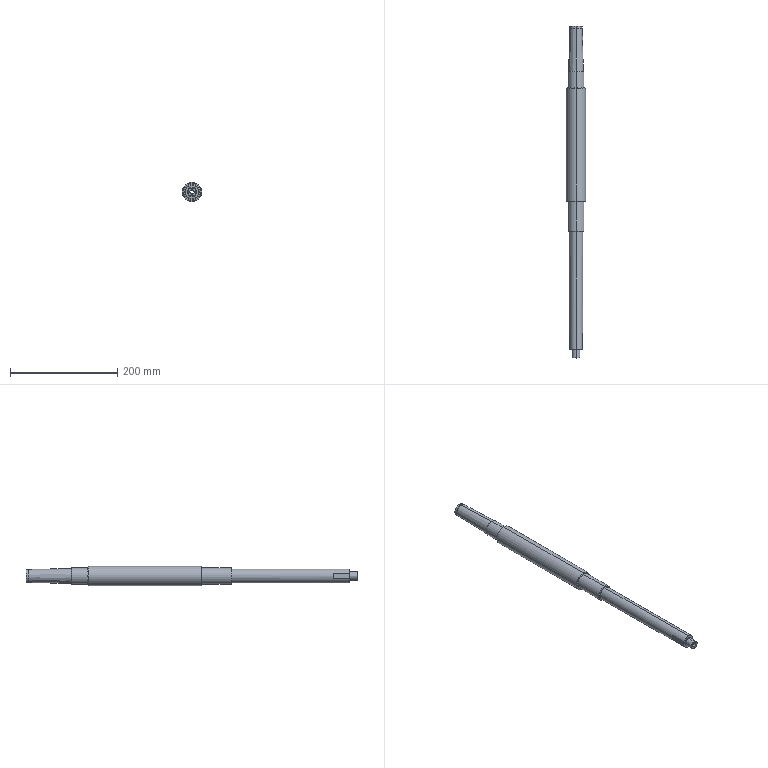Part | NX | features BREP 1 | 1 solid | 51 faces | box 36 x 618 x 36 mm | volume 396919 mm3 | cylinder 21 | plane 16 | torus 10 | cone 4 | commonest cylinder face diameters 8 x5 30 x4 14.5 x2 15 x2 22 x2 24 x2
STEP:
#1=CARTESIAN_POINT('',(0.,137.,14.975));
#2=VERTEX_POINT('',#1);
#3=CARTESIAN_POINT('',(0.,137.,-14.975));
#4=VERTEX_POINT('',#3);
#5=CARTESIAN_POINT('',(0.,137.,0.));
#6=DIRECTION('',(0.,-1.,0.));
#7=DIRECTION('',(0.,0.,-1.));
#8=AXIS2_PLACEMENT_3D('',#5,#6,#7);
#9=CIRCLE('',#8,14.975);
#10=EDGE_CURVE('',#2,#4,#9,.T.);
#11=ORIENTED_EDGE('',*,*,#10,.F.);
#12=CARTESIAN_POINT('',(0.,137.975,13.976));
#13=VERTEX_POINT('',#12);
#14=CARTESIAN_POINT('',(0.,138.,14.975));
#15=DIRECTION('',(1.,0.,0.));
#16=DIRECTION('',(0.,0.,-1.));
#17=AXIS2_PLACEMENT_3D('',#14,#15,#16);
#18=CIRCLE('',#17,1.);
#19=EDGE_CURVE('',#13,#2,#18,.F.);
#20=ORIENTED_EDGE('',*,*,#19,.F.);
#21=CARTESIAN_POINT('',(0.,137.975,-13.976));
#22=VERTEX_POINT('',#21);
#23=CARTESIAN_POINT('',(0.,137.975,0.));
#24=DIRECTION('',(0.,1.,0.));
#25=DIRECTION('',(0.,0.,-1.));
#26=AXIS2_PLACEMENT_3D('',#23,#24,#25);
#27=CIRCLE('',#26,13.976);
#28=EDGE_CURVE('',#22,#13,#27,.T.);
#29=ORIENTED_EDGE('',*,*,#28,.F.);
#30=CARTESIAN_POINT('',(0.,138.,-14.975));
#31=DIRECTION('',(-1.,0.,0.));
#32=DIRECTION('',(0.,-1.,0.));
#33=AXIS2_PLACEMENT_3D('',#30,#31,#32);
#34=CIRCLE('',#33,1.);
#35=EDGE_CURVE('',#22,#4,#34,.F.);
#36=ORIENTED_EDGE('',*,*,#35,.T.);
#37=EDGE_LOOP('',(#11,#20,#29,#36));
#38=FACE_BOUND('',#37,.T.);
#39=CARTESIAN_POINT('',(0.,138.,0.));
#40=DIRECTION('',(0.,-1.,0.));
#41=DIRECTION('',(0.,0.,1.));
#42=AXIS2_PLACEMENT_3D('',#39,#40,#41);
#43=TOROIDAL_SURFACE('',#42,14.975,1.);
#44=ADVANCED_FACE('',(#38),#43,.F.);
#45=CARTESIAN_POINT('',(0.,106.,16.));
#46=VERTEX_POINT('',#45);
#47=CARTESIAN_POINT('',(0.,106.,-16.));
#48=VERTEX_POINT('',#47);
#49=CARTESIAN_POINT('',(0.,106.,0.));
#50=DIRECTION('',(0.,-1.,0.));
#51=DIRECTION('',(0.,0.,-1.));
#52=AXIS2_PLACEMENT_3D('',#49,#50,#51);
#53=CIRCLE('',#52,16.);
#54=EDGE_CURVE('',#46,#48,#53,.T.);
#55=ORIENTED_EDGE('',*,*,#54,.F.);
#56=CARTESIAN_POINT('',(0.,107.,15.));
#57=VERTEX_POINT('',#56);
#58=CARTESIAN_POINT('',(0.,107.,16.));
#59=DIRECTION('',(1.,0.,0.));
#60=DIRECTION('',(0.,0.,-1.));
#61=AXIS2_PLACEMENT_3D('',#58,#59,#60);
#62=CIRCLE('',#61,1.);
#63=EDGE_CURVE('',#57,#46,#62,.F.);
#64=ORIENTED_EDGE('',*,*,#63,.F.);
#65=CARTESIAN_POINT('',(0.,107.,-15.));
#66=VERTEX_POINT('',#65);
#67=CARTESIAN_POINT('',(0.,107.,0.));
#68=DIRECTION('',(0.,1.,0.));
#69=DIRECTION('',(0.,0.,-1.));
#70=AXIS2_PLACEMENT_3D('',#67,#68,#69);
#71=CIRCLE('',#70,15.);
#72=EDGE_CURVE('',#66,#57,#71,.T.);
#73=ORIENTED_EDGE('',*,*,#72,.F.);
#74=CARTESIAN_POINT('',(0.,107.,-16.));
#75=DIRECTION('',(-1.,0.,0.));
#76=DIRECTION('',(0.,-1.,0.));
#77=AXIS2_PLACEMENT_3D('',#74,#75,#76);
#78=CIRCLE('',#77,1.);
#79=EDGE_CURVE('',#66,#48,#78,.F.);
#80=ORIENTED_EDGE('',*,*,#79,.T.);
#81=EDGE_LOOP('',(#55,#64,#73,#80));
#82=FACE_BOUND('',#81,.T.);
#83=CARTESIAN_POINT('',(0.,107.,0.));
#84=DIRECTION('',(0.,-1.,0.));
#85=DIRECTION('',(0.,0.,1.));
#86=AXIS2_PLACEMENT_3D('',#83,#84,#85);
#87=TOROIDAL_SURFACE('',#86,16.,1.);
#88=ADVANCED_FACE('',(#82),#87,.F.);
#89=CARTESIAN_POINT('',(0.,-104.,-16.));
#90=VERTEX_POINT('',#89);
#91=CARTESIAN_POINT('',(0.,-104.,16.));
#92=VERTEX_POINT('',#91);
#93=CARTESIAN_POINT('',(0.,-104.,0.));
#94=DIRECTION('',(0.,1.,0.));
#95=DIRECTION('',(0.,0.,1.));
#96=AXIS2_PLACEMENT_3D('',#93,#94,#95);
#97=CIRCLE('',#96,16.);
#98=EDGE_CURVE('',#90,#92,#97,.T.);
#99=ORIENTED_EDGE('',*,*,#98,.F.);
#100=CARTESIAN_POINT('',(0.,-105.,-15.));
#101=VERTEX_POINT('',#100);
#102=CARTESIAN_POINT('',(0.,-105.,-16.));
#103=DIRECTION('',(1.,0.,0.));
#104=DIRECTION('',(0.,0.,-1.));
#105=AXIS2_PLACEMENT_3D('',#102,#103,#104);
#106=CIRCLE('',#105,1.);
#107=EDGE_CURVE('',#90,#101,#106,.T.);
#108=ORIENTED_EDGE('',*,*,#107,.T.);
#109=CARTESIAN_POINT('',(0.,-105.,15.));
#110=VERTEX_POINT('',#109);
#111=CARTESIAN_POINT('',(0.,-105.,0.));
#112=DIRECTION('',(0.,-1.,0.));
#113=DIRECTION('',(0.,0.,1.));
#114=AXIS2_PLACEMENT_3D('',#111,#112,#113);
#115=CIRCLE('',#114,15.);
#116=EDGE_CURVE('',#110,#101,#115,.T.);
#117=ORIENTED_EDGE('',*,*,#116,.F.);
#118=CARTESIAN_POINT('',(0.,-105.,16.));
#119=DIRECTION('',(-1.,0.,0.));
#120=DIRECTION('',(0.,-1.,0.));
#121=AXIS2_PLACEMENT_3D('',#118,#119,#120);
#122=CIRCLE('',#121,1.);
#123=EDGE_CURVE('',#92,#110,#122,.T.);
#124=ORIENTED_EDGE('',*,*,#123,.F.);
#125=EDGE_LOOP('',(#99,#108,#117,#124));
#126=FACE_BOUND('',#125,.T.);
#127=CARTESIAN_POINT('',(0.,-105.,0.));
#128=DIRECTION('',(0.,1.,0.));
#129=DIRECTION('',(0.,0.,-1.));
#130=AXIS2_PLACEMENT_3D('',#127,#128,#129);
#131=TOROIDAL_SURFACE('',#130,16.,1.);
#132=ADVANCED_FACE('',(#126),#131,.F.);
#133=CARTESIAN_POINT('',(0.,-160.,-13.5));
#134=VERTEX_POINT('',#133);
#135=CARTESIAN_POINT('',(0.,-160.,13.5));
#136=VERTEX_POINT('',#135);
#137=CARTESIAN_POINT('',(0.,-160.,0.));
#138=DIRECTION('',(0.,1.,0.));
#139=DIRECTION('',(0.,0.,1.));
#140=AXIS2_PLACEMENT_3D('',#137,#138,#139);
#141=CIRCLE('',#140,13.5);
#142=EDGE_CURVE('',#134,#136,#141,.T.);
#143=ORIENTED_EDGE('',*,*,#142,.F.);
#144=CARTESIAN_POINT('',(0.,-161.,-12.5));
#145=VERTEX_POINT('',#144);
#146=CARTESIAN_POINT('',(0.,-161.,-13.5));
#147=DIRECTION('',(1.,0.,0.));
#148=DIRECTION('',(0.,0.,-1.));
#149=AXIS2_PLACEMENT_3D('',#146,#147,#148);
#150=CIRCLE('',#149,1.);
#151=EDGE_CURVE('',#134,#145,#150,.T.);
#152=ORIENTED_EDGE('',*,*,#151,.T.);
#153=CARTESIAN_POINT('',(0.,-161.,12.5));
#154=VERTEX_POINT('',#153);
#155=CARTESIAN_POINT('',(0.,-161.,0.));
#156=DIRECTION('',(0.,-1.,0.));
#157=DIRECTION('',(0.,0.,1.));
#158=AXIS2_PLACEMENT_3D('',#155,#156,#157);
#159=CIRCLE('',#158,12.5);
#160=EDGE_CURVE('',#154,#145,#159,.T.);
#161=ORIENTED_EDGE('',*,*,#160,.F.);
#162=CARTESIAN_POINT('',(0.,-161.,13.5));
#163=DIRECTION('',(-1.,0.,0.));
#164=DIRECTION('',(0.,-1.,0.));
#165=AXIS2_PLACEMENT_3D('',#162,#163,#164);
#166=CIRCLE('',#165,1.);
#167=EDGE_CURVE('',#136,#154,#166,.T.);
#168=ORIENTED_EDGE('',*,*,#167,.F.);
#169=EDGE_LOOP('',(#143,#152,#161,#168));
#170=FACE_BOUND('',#169,.T.);
#171=CARTESIAN_POINT('',(0.,-161.,0.));
#172=DIRECTION('',(0.,1.,0.));
#173=DIRECTION('',(0.,0.,-1.));
#174=AXIS2_PLACEMENT_3D('',#171,#172,#173);
#175=TOROIDAL_SURFACE('',#174,13.5,1.);
#176=ADVANCED_FACE('',(#170),#175,.F.);
#177=CARTESIAN_POINT('',(0.,-380.,-8.5));
#178=VERTEX_POINT('',#177);
#179=CARTESIAN_POINT('',(0.,-380.,8.5));
#180=VERTEX_POINT('',#179);
#181=CARTESIAN_POINT('',(0.,-380.,0.));
#182=DIRECTION('',(0.,1.,0.));
#183=DIRECTION('',(0.,0.,1.));
#184=AXIS2_PLACEMENT_3D('',#181,#182,#183);
#185=CIRCLE('',#184,8.5);
#186=EDGE_CURVE('',#178,#180,#185,.T.);
#187=ORIENTED_EDGE('',*,*,#186,.F.);
#188=CARTESIAN_POINT('',(0.,-381.,-7.5));
#189=VERTEX_POINT('',#188);
#190=CARTESIAN_POINT('',(0.,-381.,-8.5));
#191=DIRECTION('',(1.,0.,0.));
#192=DIRECTION('',(0.,0.,-1.));
#193=AXIS2_PLACEMENT_3D('',#190,#191,#192);
#194=CIRCLE('',#193,1.);
#195=EDGE_CURVE('',#178,#189,#194,.T.);
#196=ORIENTED_EDGE('',*,*,#195,.T.);
#197=CARTESIAN_POINT('',(0.,-381.,7.5));
#198=VERTEX_POINT('',#197);
#199=CARTESIAN_POINT('',(0.,-381.,0.));
#200=DIRECTION('',(0.,-1.,0.));
#201=DIRECTION('',(0.,0.,1.));
#202=AXIS2_PLACEMENT_3D('',#199,#200,#201);
#203=CIRCLE('',#202,7.5);
#204=EDGE_CURVE('',#198,#189,#203,.T.);
#205=ORIENTED_EDGE('',*,*,#204,.F.);
#206=CARTESIAN_POINT('',(0.,-381.,8.5));
#207=DIRECTION('',(-1.,0.,0.));
#208=DIRECTION('',(0.,-1.,0.));
#209=AXIS2_PLACEMENT_3D('',#206,#207,#208);
#210=CIRCLE('',#209,1.);
#211=EDGE_CURVE('',#180,#198,#210,.T.);
#212=ORIENTED_EDGE('',*,*,#211,.F.);
#213=EDGE_LOOP('',(#187,#196,#205,#212));
#214=FACE_BOUND('',#213,.T.);
#215=CARTESIAN_POINT('',(0.,-381.,0.));
#216=DIRECTION('',(0.,1.,0.));
#217=DIRECTION('',(0.,0.,-1.));
#218=AXIS2_PLACEMENT_3D('',#215,#216,#217);
#219=TOROIDAL_SURFACE('',#218,8.5,1.);
#220=ADVANCED_FACE('',(#214),#219,.F.);
#221=CARTESIAN_POINT('',(12.763,162.,4.));
#222=VERTEX_POINT('',#221);
#223=CARTESIAN_POINT('',(13.475,158.,0.));
#224=VERTEX_POINT('',#223);
#225=CARTESIAN_POINT('',(12.763,162.,4.));
#226=CARTESIAN_POINT('',(12.791,160.935,4.));
#227=CARTESIAN_POINT('',(13.156,158.88,3.129));
#228=CARTESIAN_POINT('',(13.475,158.,1.065));
#229=CARTESIAN_POINT('',(13.475,158.,0.));
#230=B_SPLINE_CURVE_WITH_KNOTS('',3,(#225,#226,#227,#228,#229),.UNSPECIFIED.,.F.,.F.,(4,1,4),(0.,0.003148,0.006296),.UNSPECIFIED.);
#231=EDGE_CURVE('',#222,#224,#230,.T.);
#232=ORIENTED_EDGE('',*,*,#231,.T.);
#233=CARTESIAN_POINT('',(8.4,158.,0.));
#234=VERTEX_POINT('',#233);
#235=CARTESIAN_POINT('',(21.,158.,0.));
#236=DIRECTION('',(-1.,0.,0.));
#237=VECTOR('',#236,1000.);
#238=LINE('',#235,#237);
#239=EDGE_CURVE('',#224,#234,#238,.T.);
#240=ORIENTED_EDGE('',*,*,#239,.T.);
#241=CARTESIAN_POINT('',(8.4,162.,4.));
#242=VERTEX_POINT('',#241);
#243=CARTESIAN_POINT('',(8.4,162.,0.));
#244=DIRECTION('',(1.,0.,0.));
#245=DIRECTION('',(0.,1.,0.));
#246=AXIS2_PLACEMENT_3D('',#243,#244,#245);
#247=CIRCLE('',#246,4.);
#248=EDGE_CURVE('',#242,#234,#247,.T.);
#249=ORIENTED_EDGE('',*,*,#248,.F.);
#250=CARTESIAN_POINT('',(11.,162.,4.));
#251=DIRECTION('',(1.,0.,0.));
#252=VECTOR('',#251,1000.);
#253=LINE('',#250,#252);
#254=EDGE_CURVE('',#242,#222,#253,.T.);
#255=ORIENTED_EDGE('',*,*,#254,.T.);
#256=EDGE_LOOP('',(#232,#240,#249,#255));
#257=FACE_BOUND('',#256,.T.);
#258=CARTESIAN_POINT('',(21.,162.,0.));
#259=DIRECTION('',(-1.,0.,0.));
#260=DIRECTION('',(0.,1.,0.));
#261=AXIS2_PLACEMENT_3D('',#258,#259,#260);
#262=CYLINDRICAL_SURFACE('',#261,4.);
#263=ADVANCED_FACE('',(#257),#262,.F.);
#264=CARTESIAN_POINT('',(0.,217.,11.));
#265=VERTEX_POINT('',#264);
#266=CARTESIAN_POINT('',(0.,217.,-11.));
#267=VERTEX_POINT('',#266);
#268=CARTESIAN_POINT('',(0.,217.,0.));
#269=DIRECTION('',(0.,1.,0.));
#270=DIRECTION('',(0.,0.,1.));
#271=AXIS2_PLACEMENT_3D('',#268,#269,#270);
#272=CIRCLE('',#271,11.);
#273=EDGE_CURVE('',#265,#267,#272,.T.);
#274=ORIENTED_EDGE('',*,*,#273,.T.);
#275=CARTESIAN_POINT('',(0.,218.,-11.));
#276=VERTEX_POINT('',#275);
#277=CARTESIAN_POINT('',(0.,217.,-11.));
#278=DIRECTION('',(0.,1.,0.));
#279=VECTOR('',#278,1000.);
#280=LINE('',#277,#279);
#281=EDGE_CURVE('',#267,#276,#280,.T.);
#282=ORIENTED_EDGE('',*,*,#281,.T.);
#283=CARTESIAN_POINT('',(0.,218.,11.));
#284=VERTEX_POINT('',#283);
#285=CARTESIAN_POINT('',(0.,218.,0.));
#286=DIRECTION('',(0.,1.,0.));
#287=DIRECTION('',(0.,0.,1.));
#288=AXIS2_PLACEMENT_3D('',#285,#286,#287);
#289=CIRCLE('',#288,11.);
#290=EDGE_CURVE('',#284,#276,#289,.T.);
#291=ORIENTED_EDGE('',*,*,#290,.F.);
#292=CARTESIAN_POINT('',(0.,217.,11.));
#293=DIRECTION('',(0.,1.,0.));
#294=VECTOR('',#293,1000.);
#295=LINE('',#292,#294);
#296=EDGE_CURVE('',#265,#284,#295,.T.);
#297=ORIENTED_EDGE('',*,*,#296,.F.);
#298=EDGE_LOOP('',(#274,#282,#291,#297));
#299=FACE_BOUND('',#298,.T.);
#300=CARTESIAN_POINT('',(0.,217.,0.));
#301=DIRECTION('',(0.,1.,0.));
#302=DIRECTION('',(0.,0.,-1.));
#303=AXIS2_PLACEMENT_3D('',#300,#301,#302);
#304=CYLINDRICAL_SURFACE('',#303,11.);
#305=ADVANCED_FACE('',(#299),#304,.T.);
#306=CARTESIAN_POINT('',(0.,212.,-8.038));
#307=VERTEX_POINT('',#306);
#308=CARTESIAN_POINT('',(0.,212.,6.462));
#309=VERTEX_POINT('',#308);
#310=CARTESIAN_POINT('',(0.,212.,-0.7881));
#311=DIRECTION('',(0.,1.,0.));
#312=DIRECTION('',(0.,0.,1.));
#313=AXIS2_PLACEMENT_3D('',#310,#311,#312);
#314=CIRCLE('',#313,7.25);
#315=EDGE_CURVE('',#307,#309,#314,.T.);
#316=ORIENTED_EDGE('',*,*,#315,.F.);
#317=CARTESIAN_POINT('',(0.,222.,-8.038));
#318=VERTEX_POINT('',#317);
#319=CARTESIAN_POINT('',(0.,222.,-8.038));
#320=DIRECTION('',(0.,1.,0.));
#321=VECTOR('',#320,1000.);
#322=LINE('',#319,#321);
#323=EDGE_CURVE('',#307,#318,#322,.T.);
#324=ORIENTED_EDGE('',*,*,#323,.T.);
#325=CARTESIAN_POINT('',(0.,222.,6.462));
#326=VERTEX_POINT('',#325);
#327=CARTESIAN_POINT('',(0.,222.,-0.7881));
#328=DIRECTION('',(0.,1.,0.));
#329=DIRECTION('',(0.,0.,1.));
#330=AXIS2_PLACEMENT_3D('',#327,#328,#329);
#331=CIRCLE('',#330,7.25);
#332=EDGE_CURVE('',#318,#326,#331,.T.);
#333=ORIENTED_EDGE('',*,*,#332,.T.);
#334=CARTESIAN_POINT('',(0.,222.,6.462));
#335=DIRECTION('',(0.,1.,0.));
#336=VECTOR('',#335,1000.);
#337=LINE('',#334,#336);
#338=EDGE_CURVE('',#309,#326,#337,.T.);
#339=ORIENTED_EDGE('',*,*,#338,.F.);
#340=EDGE_LOOP('',(#316,#324,#333,#339));
#341=FACE_BOUND('',#340,.T.);
#342=CARTESIAN_POINT('',(0.,222.,-0.7881));
#343=DIRECTION('',(0.,1.,0.));
#344=DIRECTION('',(0.,0.,-1.));
#345=AXIS2_PLACEMENT_3D('',#342,#343,#344);
#346=CYLINDRICAL_SURFACE('',#345,7.25);
#347=ADVANCED_FACE('',(#341),#346,.F.);
#348=CARTESIAN_POINT('',(0.,209.574,-4.));
#349=VERTEX_POINT('',#348);
#350=CARTESIAN_POINT('',(0.,210.521,4.));
#351=VERTEX_POINT('',#350);
#352=CARTESIAN_POINT('',(0.,209.574,-4.));
#353=CARTESIAN_POINT('',(-1.061,209.574,-4.));
#354=CARTESIAN_POINT('',(-3.135,209.707,-3.125));
#355=CARTESIAN_POINT('',(-4.431,210.103,-0.008504));
#356=CARTESIAN_POINT('',(-3.141,210.436,3.124));
#357=CARTESIAN_POINT('',(-1.061,210.521,4.));
#358=CARTESIAN_POINT('',(0.,210.521,4.));
#359=B_SPLINE_CURVE_WITH_KNOTS('',3,(#352,#353,#354,#355,#356,#357,#358),.UNSPECIFIED.,.F.,.F.,(4,1,1,1,4),(0.,0.003137,0.006274,0.009411,0.01255),.UNSPECIFIED.);
#360=EDGE_CURVE('',#349,#351,#359,.T.);
#361=ORIENTED_EDGE('',*,*,#360,.F.);
#362=CARTESIAN_POINT('',(0.,212.,-8.038));
#363=DIRECTION('',(0.,0.515,-0.8572));
#364=VECTOR('',#363,1000.);
#365=LINE('',#362,#364);
#366=EDGE_CURVE('',#349,#307,#365,.T.);
#367=ORIENTED_EDGE('',*,*,#366,.T.);
#368=ORIENTED_EDGE('',*,*,#315,.T.);
#369=CARTESIAN_POINT('',(0.,212.,6.462));
#370=DIRECTION('',(0.,0.515,0.8572));
#371=VECTOR('',#370,1000.);
#372=LINE('',#369,#371);
#373=EDGE_CURVE('',#351,#309,#372,.T.);
#374=ORIENTED_EDGE('',*,*,#373,.F.);
#375=EDGE_LOOP('',(#361,#367,#368,#374));
#376=FACE_BOUND('',#375,.T.);
#377=CARTESIAN_POINT('',(0.,212.,-0.7881));
#378=DIRECTION('',(0.,1.,0.));
#379=DIRECTION('',(0.,0.,-1.));
#380=AXIS2_PLACEMENT_3D('',#377,#378,#379);
#381=CONICAL_SURFACE('',#380,7.25,1.03);
#382=ADVANCED_FACE('',(#376),#381,.F.);
#383=CARTESIAN_POINT('',(0.,137.,-15.));
#384=VERTEX_POINT('',#383);
#385=CARTESIAN_POINT('',(0.,137.,15.));
#386=VERTEX_POINT('',#385);
#387=CARTESIAN_POINT('',(0.,137.,0.));
#388=DIRECTION('',(0.,-1.,0.));
#389=DIRECTION('',(0.,0.,-1.));
#390=AXIS2_PLACEMENT_3D('',#387,#388,#389);
#391=CIRCLE('',#390,15.);
#392=EDGE_CURVE('',#384,#386,#391,.T.);
#393=ORIENTED_EDGE('',*,*,#392,.T.);
#394=CARTESIAN_POINT('',(0.,0.,15.));
#395=DIRECTION('',(0.,-1.,0.));
#396=VECTOR('',#395,1000.);
#397=LINE('',#394,#396);
#398=EDGE_CURVE('',#57,#386,#397,.F.);
#399=ORIENTED_EDGE('',*,*,#398,.F.);
#400=CARTESIAN_POINT('',(0.,107.,0.));
#401=DIRECTION('',(0.,1.,0.));
#402=DIRECTION('',(0.,0.,-1.));
#403=AXIS2_PLACEMENT_3D('',#400,#401,#402);
#404=CIRCLE('',#403,15.);
#405=EDGE_CURVE('',#57,#66,#404,.T.);
#406=ORIENTED_EDGE('',*,*,#405,.T.);
#407=CARTESIAN_POINT('',(0.,0.,-15.));
#408=DIRECTION('',(0.,-1.,0.));
#409=VECTOR('',#408,1000.);
#410=LINE('',#407,#409);
#411=EDGE_CURVE('',#66,#384,#410,.F.);
#412=ORIENTED_EDGE('',*,*,#411,.T.);
#413=EDGE_LOOP('',(#393,#399,#406,#412));
#414=FACE_BOUND('',#413,.T.);
#415=CARTESIAN_POINT('',(0.,0.,0.));
#416=DIRECTION('',(0.,-1.,0.));
#417=DIRECTION('',(0.,0.,1.));
#418=AXIS2_PLACEMENT_3D('',#415,#416,#417);
#419=CYLINDRICAL_SURFACE('',#418,15.);
#420=ADVANCED_FACE('',(#414),#419,.T.);
#421=CARTESIAN_POINT('',(0.,222.,-12.));
#422=VERTEX_POINT('',#421);
#423=CARTESIAN_POINT('',(0.,222.,12.));
#424=VERTEX_POINT('',#423);
#425=CARTESIAN_POINT('',(0.,222.,0.));
#426=DIRECTION('',(0.,-1.,0.));
#427=DIRECTION('',(0.,0.,-1.));
#428=AXIS2_PLACEMENT_3D('',#425,#426,#427);
#429=CIRCLE('',#428,12.);
#430=EDGE_CURVE('',#422,#424,#429,.T.);
#431=ORIENTED_EDGE('',*,*,#430,.T.);
#432=CARTESIAN_POINT('',(0.,218.,12.));
#433=VERTEX_POINT('',#432);
#434=CARTESIAN_POINT('',(0.,0.,12.));
#435=DIRECTION('',(0.,-1.,0.));
#436=VECTOR('',#435,1000.);
#437=LINE('',#434,#436);
#438=EDGE_CURVE('',#433,#424,#437,.F.);
#439=ORIENTED_EDGE('',*,*,#438,.F.);
#440=CARTESIAN_POINT('',(0.,218.,-12.));
#441=VERTEX_POINT('',#440);
#442=CARTESIAN_POINT('',(0.,218.,0.));
#443=DIRECTION('',(0.,1.,0.));
#444=DIRECTION('',(0.,0.,1.));
#445=AXIS2_PLACEMENT_3D('',#442,#443,#444);
#446=CIRCLE('',#445,12.);
#447=EDGE_CURVE('',#433,#441,#446,.T.);
#448=ORIENTED_EDGE('',*,*,#447,.T.);
#449=CARTESIAN_POINT('',(0.,0.,-12.));
#450=DIRECTION('',(0.,-1.,0.));
#451=VECTOR('',#450,1000.);
#452=LINE('',#449,#451);
#453=EDGE_CURVE('',#441,#422,#452,.F.);
#454=ORIENTED_EDGE('',*,*,#453,.T.);
#455=EDGE_LOOP('',(#431,#439,#448,#454));
#456=FACE_BOUND('',#455,.T.);
#457=CARTESIAN_POINT('',(0.,0.,0.));
#458=DIRECTION('',(0.,-1.,0.));
#459=DIRECTION('',(0.,0.,1.));
#460=AXIS2_PLACEMENT_3D('',#457,#458,#459);
#461=CYLINDRICAL_SURFACE('',#460,12.);
#462=ADVANCED_FACE('',(#456),#461,.T.);
#463=ORIENTED_EDGE('',*,*,#360,.T.);
#464=CARTESIAN_POINT('',(0.,-396.,4.));
#465=VERTEX_POINT('',#464);
#466=CARTESIAN_POINT('',(0.,0.,4.));
#467=DIRECTION('',(0.,-1.,0.));
#468=VECTOR('',#467,1000.);
#469=LINE('',#466,#468);
#470=EDGE_CURVE('',#465,#351,#469,.F.);
#471=ORIENTED_EDGE('',*,*,#470,.F.);
#472=CARTESIAN_POINT('',(0.,-396.,-4.));
#473=VERTEX_POINT('',#472);
#474=CARTESIAN_POINT('',(0.,-396.,0.));
#475=DIRECTION('',(0.,-1.,0.));
#476=DIRECTION('',(0.,0.,-1.));
#477=AXIS2_PLACEMENT_3D('',#474,#475,#476);
#478=CIRCLE('',#477,4.);
#479=EDGE_CURVE('',#465,#473,#478,.T.);
#480=ORIENTED_EDGE('',*,*,#479,.T.);
#481=CARTESIAN_POINT('',(0.,0.,-4.));
#482=DIRECTION('',(0.,-1.,0.));
#483=VECTOR('',#482,1000.);
#484=LINE('',#481,#483);
#485=EDGE_CURVE('',#473,#349,#484,.F.);
#486=ORIENTED_EDGE('',*,*,#485,.T.);
#487=EDGE_LOOP('',(#463,#471,#480,#486));
#488=FACE_BOUND('',#487,.T.);
#489=CARTESIAN_POINT('',(0.,0.,0.));
#490=DIRECTION('',(0.,-1.,0.));
#491=DIRECTION('',(0.,0.,1.));
#492=AXIS2_PLACEMENT_3D('',#489,#490,#491);
#493=CYLINDRICAL_SURFACE('',#492,4.);
#494=ADVANCED_FACE('',(#488),#493,.F.);
#495=CARTESIAN_POINT('',(0.,-381.,0.));
#496=DIRECTION('',(0.,-1.,0.));
#497=DIRECTION('',(0.,0.,1.));
#498=AXIS2_PLACEMENT_3D('',#495,#496,#497);
#499=CIRCLE('',#498,7.5);
#500=EDGE_CURVE('',#189,#198,#499,.T.);
#501=ORIENTED_EDGE('',*,*,#500,.T.);
#502=CARTESIAN_POINT('',(0.,-396.,7.5));
#503=VERTEX_POINT('',#502);
#504=CARTESIAN_POINT('',(0.,0.,7.5));
#505=DIRECTION('',(0.,-1.,0.));
#506=VECTOR('',#505,1000.);
#507=LINE('',#504,#506);
#508=EDGE_CURVE('',#503,#198,#507,.F.);
#509=ORIENTED_EDGE('',*,*,#508,.F.);
#510=CARTESIAN_POINT('',(0.,-396.,-7.5));
#511=VERTEX_POINT('',#510);
#512=CARTESIAN_POINT('',(0.,-396.,0.));
#513=DIRECTION('',(0.,-1.,0.));
#514=DIRECTION('',(0.,0.,-1.));
#515=AXIS2_PLACEMENT_3D('',#512,#513,#514);
#516=CIRCLE('',#515,7.5);
#517=EDGE_CURVE('',#511,#503,#516,.T.);
#518=ORIENTED_EDGE('',*,*,#517,.F.);
#519=CARTESIAN_POINT('',(0.,0.,-7.5));
#520=DIRECTION('',(0.,-1.,0.));
#521=VECTOR('',#520,1000.);
#522=LINE('',#519,#521);
#523=EDGE_CURVE('',#511,#189,#522,.F.);
#524=ORIENTED_EDGE('',*,*,#523,.T.);
#525=EDGE_LOOP('',(#501,#509,#518,#524));
#526=FACE_BOUND('',#525,.T.);
#527=CARTESIAN_POINT('',(0.,0.,0.));
#528=DIRECTION('',(0.,-1.,0.));
#529=DIRECTION('',(0.,0.,1.));
#530=AXIS2_PLACEMENT_3D('',#527,#528,#529);
#531=CYLINDRICAL_SURFACE('',#530,7.5);
#532=ADVANCED_FACE('',(#526),#531,.T.);
#533=CARTESIAN_POINT('',(0.,-105.,0.));
#534=DIRECTION('',(0.,-1.,0.));
#535=DIRECTION('',(0.,0.,1.));
#536=AXIS2_PLACEMENT_3D('',#533,#534,#535);
#537=CIRCLE('',#536,15.);
#538=EDGE_CURVE('',#101,#110,#537,.T.);
#539=ORIENTED_EDGE('',*,*,#538,.T.);
#540=CARTESIAN_POINT('',(0.,-160.,15.));
#541=VERTEX_POINT('',#540);
#542=CARTESIAN_POINT('',(0.,0.,15.));
#543=DIRECTION('',(0.,-1.,0.));
#544=VECTOR('',#543,1000.);
#545=LINE('',#542,#544);
#546=EDGE_CURVE('',#541,#110,#545,.F.);
#547=ORIENTED_EDGE('',*,*,#546,.F.);
#548=CARTESIAN_POINT('',(0.,-160.,-15.));
#549=VERTEX_POINT('',#548);
#550=CARTESIAN_POINT('',(0.,-160.,0.));
#551=DIRECTION('',(0.,-1.,0.));
#552=DIRECTION('',(0.,0.,-1.));
#553=AXIS2_PLACEMENT_3D('',#550,#551,#552);
#554=CIRCLE('',#553,15.);
#555=EDGE_CURVE('',#549,#541,#554,.T.);
#556=ORIENTED_EDGE('',*,*,#555,.F.);
#557=CARTESIAN_POINT('',(0.,0.,-15.));
#558=DIRECTION('',(0.,-1.,0.));
#559=VECTOR('',#558,1000.);
#560=LINE('',#557,#559);
#561=EDGE_CURVE('',#549,#101,#560,.F.);
#562=ORIENTED_EDGE('',*,*,#561,.T.);
#563=EDGE_LOOP('',(#539,#547,#556,#562));
#564=FACE_BOUND('',#563,.T.);
#565=CARTESIAN_POINT('',(0.,0.,0.));
#566=DIRECTION('',(0.,-1.,0.));
#567=DIRECTION('',(0.,0.,1.));
#568=AXIS2_PLACEMENT_3D('',#565,#566,#567);
#569=CYLINDRICAL_SURFACE('',#568,15.);
#570=ADVANCED_FACE('',(#564),#569,.T.);
#571=CARTESIAN_POINT('',(0.,106.,-18.));
#572=VERTEX_POINT('',#571);
#573=CARTESIAN_POINT('',(0.,106.,18.));
#574=VERTEX_POINT('',#573);
#575=CARTESIAN_POINT('',(0.,106.,0.));
#576=DIRECTION('',(0.,-1.,0.));
#577=DIRECTION('',(0.,0.,-1.));
#578=AXIS2_PLACEMENT_3D('',#575,#576,#577);
#579=CIRCLE('',#578,18.);
#580=EDGE_CURVE('',#572,#574,#579,.T.);
#581=ORIENTED_EDGE('',*,*,#580,.T.);
#582=CARTESIAN_POINT('',(0.,-104.,18.));
#583=VERTEX_POINT('',#582);
#584=CARTESIAN_POINT('',(0.,0.,18.));
#585=DIRECTION('',(0.,-1.,0.));
#586=VECTOR('',#585,1000.);
#587=LINE('',#584,#586);
#588=EDGE_CURVE('',#583,#574,#587,.F.);
#589=ORIENTED_EDGE('',*,*,#588,.F.);
#590=CARTESIAN_POINT('',(0.,-104.,-18.));
#591=VERTEX_POINT('',#590);
#592=CARTESIAN_POINT('',(0.,-104.,0.));
#593=DIRECTION('',(0.,-1.,0.));
#594=DIRECTION('',(0.,0.,-1.));
#595=AXIS2_PLACEMENT_3D('',#592,#593,#594);
#596=CIRCLE('',#595,18.);
#597=EDGE_CURVE('',#591,#583,#596,.T.);
#598=ORIENTED_EDGE('',*,*,#597,.F.);
#599=CARTESIAN_POINT('',(0.,0.,-18.));
#600=DIRECTION('',(0.,-1.,0.));
#601=VECTOR('',#600,1000.);
#602=LINE('',#599,#601);
#603=EDGE_CURVE('',#591,#572,#602,.F.);
#604=ORIENTED_EDGE('',*,*,#603,.T.);
#605=EDGE_LOOP('',(#581,#589,#598,#604));
#606=FACE_BOUND('',#605,.T.);
#607=CARTESIAN_POINT('',(0.,0.,0.));
#608=DIRECTION('',(0.,-1.,0.));
#609=DIRECTION('',(0.,0.,1.));
#610=AXIS2_PLACEMENT_3D('',#607,#608,#609);
#611=CYLINDRICAL_SURFACE('',#610,18.);
#612=ADVANCED_FACE('',(#606),#611,.T.);
#613=CARTESIAN_POINT('',(0.,-161.,0.));
#614=DIRECTION('',(0.,-1.,0.));
#615=DIRECTION('',(0.,0.,1.));
#616=AXIS2_PLACEMENT_3D('',#613,#614,#615);
#617=CIRCLE('',#616,12.5);
#618=EDGE_CURVE('',#145,#154,#617,.T.);
#619=ORIENTED_EDGE('',*,*,#618,.T.);
#620=CARTESIAN_POINT('',(0.,-380.,12.5));
#621=VERTEX_POINT('',#620);
#622=CARTESIAN_POINT('',(0.,0.,12.5));
#623=DIRECTION('',(0.,-1.,0.));
#624=VECTOR('',#623,1000.);
#625=LINE('',#622,#624);
#626=EDGE_CURVE('',#621,#154,#625,.F.);
#627=ORIENTED_EDGE('',*,*,#626,.F.);
#628=CARTESIAN_POINT('',(11.5,-380.,4.899));
#629=VERTEX_POINT('',#628);
#630=CARTESIAN_POINT('',(0.,-380.,0.));
#631=DIRECTION('',(0.,-1.,0.));
#632=DIRECTION('',(0.,0.,-1.));
#633=AXIS2_PLACEMENT_3D('',#630,#631,#632);
#634=CIRCLE('',#633,12.5);
#635=EDGE_CURVE('',#629,#621,#634,.T.);
#636=ORIENTED_EDGE('',*,*,#635,.F.);
#637=CARTESIAN_POINT('',(11.5,-350.,4.899));
#638=VERTEX_POINT('',#637);
#639=CARTESIAN_POINT('',(11.5,0.,4.899));
#640=DIRECTION('',(0.,-1.,0.));
#641=VECTOR('',#640,1000.);
#642=LINE('',#639,#641);
#643=EDGE_CURVE('',#638,#629,#642,.T.);
#644=ORIENTED_EDGE('',*,*,#643,.F.);
#645=CARTESIAN_POINT('',(11.5,-350.,-4.899));
#646=VERTEX_POINT('',#645);
#647=CARTESIAN_POINT('',(0.,-350.,0.));
#648=DIRECTION('',(0.,-1.,0.));
#649=DIRECTION('',(0.,0.,-1.));
#650=AXIS2_PLACEMENT_3D('',#647,#648,#649);
#651=CIRCLE('',#650,12.5);
#652=EDGE_CURVE('',#646,#638,#651,.T.);
#653=ORIENTED_EDGE('',*,*,#652,.F.);
#654=CARTESIAN_POINT('',(11.5,-380.,-4.899));
#655=VERTEX_POINT('',#654);
#656=CARTESIAN_POINT('',(11.5,0.,-4.899));
#657=DIRECTION('',(0.,1.,0.));
#658=VECTOR('',#657,1000.);
#659=LINE('',#656,#658);
#660=EDGE_CURVE('',#655,#646,#659,.T.);
#661=ORIENTED_EDGE('',*,*,#660,.F.);
#662=CARTESIAN_POINT('',(0.,-380.,-12.5));
#663=VERTEX_POINT('',#662);
#664=CARTESIAN_POINT('',(0.,-380.,0.));
#665=DIRECTION('',(0.,-1.,0.));
#666=DIRECTION('',(0.,0.,-1.));
#667=AXIS2_PLACEMENT_3D('',#664,#665,#666);
#668=CIRCLE('',#667,12.5);
#669=EDGE_CURVE('',#663,#655,#668,.T.);
#670=ORIENTED_EDGE('',*,*,#669,.F.);
#671=CARTESIAN_POINT('',(0.,0.,-12.5));
#672=DIRECTION('',(0.,-1.,0.));
#673=VECTOR('',#672,1000.);
#674=LINE('',#671,#673);
#675=EDGE_CURVE('',#663,#145,#674,.F.);
#676=ORIENTED_EDGE('',*,*,#675,.T.);
#677=EDGE_LOOP('',(#619,#627,#636,#644,#653,#661,#670,#676));
#678=FACE_BOUND('',#677,.T.);
#679=CARTESIAN_POINT('',(0.,0.,0.));
#680=DIRECTION('',(0.,-1.,0.));
#681=DIRECTION('',(0.,0.,1.));
#682=AXIS2_PLACEMENT_3D('',#679,#680,#681);
#683=CYLINDRICAL_SURFACE('',#682,12.5);
#684=ADVANCED_FACE('',(#678),#683,.T.);
#685=CARTESIAN_POINT('',(0.,217.,12.));
#686=VERTEX_POINT('',#685);
#687=CARTESIAN_POINT('',(0.,217.,-12.));
#688=VERTEX_POINT('',#687);
#689=CARTESIAN_POINT('',(0.,217.,0.));
#690=DIRECTION('',(0.,1.,0.));
#691=DIRECTION('',(0.,0.,1.));
#692=AXIS2_PLACEMENT_3D('',#689,#690,#691);
#693=CIRCLE('',#692,12.);
#694=EDGE_CURVE('',#686,#688,#693,.T.);
#695=ORIENTED_EDGE('',*,*,#694,.F.);
#696=CARTESIAN_POINT('',(0.,217.,12.));
#697=DIRECTION('',(0.,-0.9997,0.02499));
#698=VECTOR('',#697,1000.);
#699=LINE('',#696,#698);
#700=EDGE_CURVE('',#13,#686,#699,.F.);
#701=ORIENTED_EDGE('',*,*,#700,.F.);
#702=CARTESIAN_POINT('',(0.,137.975,0.));
#703=DIRECTION('',(0.,1.,0.));
#704=DIRECTION('',(0.,0.,-1.));
#705=AXIS2_PLACEMENT_3D('',#702,#703,#704);
#706=CIRCLE('',#705,13.976);
#707=EDGE_CURVE('',#13,#22,#706,.T.);
#708=ORIENTED_EDGE('',*,*,#707,.T.);
#709=CARTESIAN_POINT('',(0.,217.,-12.));
#710=DIRECTION('',(0.,-0.9997,-0.02499));
#711=VECTOR('',#710,1000.);
#712=LINE('',#709,#711);
#713=EDGE_CURVE('',#22,#688,#712,.F.);
#714=ORIENTED_EDGE('',*,*,#713,.T.);
#715=EDGE_LOOP('',(#695,#701,#708,#714));
#716=FACE_BOUND('',#715,.T.);
#717=CARTESIAN_POINT('',(11.975,192.,-4.));
#718=VERTEX_POINT('',#717);
#719=CARTESIAN_POINT('',(11.975,192.,4.));
#720=VERTEX_POINT('',#719);
#721=CARTESIAN_POINT('',(11.975,192.,-4.));
#722=CARTESIAN_POINT('',(11.947,193.062,-4.));
#723=CARTESIAN_POINT('',(12.228,195.128,-3.131));
#724=CARTESIAN_POINT('',(12.674,196.436,-0.006148));
#725=CARTESIAN_POINT('',(12.228,195.129,3.133));
#726=CARTESIAN_POINT('',(11.947,193.062,4.));
#727=CARTESIAN_POINT('',(11.975,192.,4.));
#728=B_SPLINE_CURVE_WITH_KNOTS('',3,(#721,#722,#723,#724,#725,#726,#727),.UNSPECIFIED.,.F.,.F.,(4,1,1,1,4),(0.,0.003141,0.006282,0.009423,0.01256),.UNSPECIFIED.);
#729=EDGE_CURVE('',#718,#720,#728,.T.);
#730=ORIENTED_EDGE('',*,*,#729,.F.);
#731=CARTESIAN_POINT('',(12.763,162.,-4.));
#732=VERTEX_POINT('',#731);
#733=CARTESIAN_POINT('',(12.763,162.,-4.));
#734=CARTESIAN_POINT('',(12.501,172.,-4.));
#735=CARTESIAN_POINT('',(12.238,182.,-4.));
#736=CARTESIAN_POINT('',(11.975,192.,-4.));
#737=B_SPLINE_CURVE_WITH_KNOTS('',3,(#733,#734,#735,#736),.UNSPECIFIED.,.F.,.F.,(4,4),(0.,1.),.PIECEWISE_BEZIER_KNOTS.);
#738=EDGE_CURVE('',#732,#718,#737,.T.);
#739=ORIENTED_EDGE('',*,*,#738,.F.);
#740=CARTESIAN_POINT('',(13.475,158.,0.));
#741=CARTESIAN_POINT('',(13.475,158.,-1.065));
#742=CARTESIAN_POINT('',(13.156,158.877,-3.126));
#743=CARTESIAN_POINT('',(12.791,160.936,-4.));
#744=CARTESIAN_POINT('',(12.763,162.,-4.));
#745=B_SPLINE_CURVE_WITH_KNOTS('',3,(#740,#741,#742,#743,#744),.UNSPECIFIED.,.F.,.F.,(4,1,4),(0.,0.003148,0.006296),.UNSPECIFIED.);
#746=EDGE_CURVE('',#224,#732,#745,.T.);
#747=ORIENTED_EDGE('',*,*,#746,.F.);
#748=ORIENTED_EDGE('',*,*,#231,.F.);
#749=CARTESIAN_POINT('',(12.763,162.,4.));
#750=CARTESIAN_POINT('',(12.501,172.,4.));
#751=CARTESIAN_POINT('',(12.238,182.,4.));
#752=CARTESIAN_POINT('',(11.975,192.,4.));
#753=B_SPLINE_CURVE_WITH_KNOTS('',3,(#749,#750,#751,#752),.UNSPECIFIED.,.F.,.F.,(4,4),(0.,1.),.PIECEWISE_BEZIER_KNOTS.);
#754=EDGE_CURVE('',#222,#720,#753,.T.);
#755=ORIENTED_EDGE('',*,*,#754,.T.);
#756=EDGE_LOOP('',(#730,#739,#747,#748,#755));
#757=FACE_BOUND('',#756,.T.);
#758=CARTESIAN_POINT('',(0.,217.,0.));
#759=DIRECTION('',(0.,-1.,0.));
#760=DIRECTION('',(0.,0.,1.));
#761=AXIS2_PLACEMENT_3D('',#758,#759,#760);
#762=CONICAL_SURFACE('',#761,12.,0.02499);
#763=ADVANCED_FACE('',(#716,#757),#762,.T.);
#764=ORIENTED_EDGE('',*,*,#700,.T.);
#765=CARTESIAN_POINT('',(0.,217.,0.));
#766=DIRECTION('',(0.,1.,0.));
#767=DIRECTION('',(0.,0.,1.));
#768=AXIS2_PLACEMENT_3D('',#765,#766,#767);
#769=CIRCLE('',#768,12.);
#770=EDGE_CURVE('',#688,#686,#769,.T.);
#771=ORIENTED_EDGE('',*,*,#770,.F.);
#772=ORIENTED_EDGE('',*,*,#713,.F.);
#773=ORIENTED_EDGE('',*,*,#28,.T.);
#774=EDGE_LOOP('',(#764,#771,#772,#773));
#775=FACE_BOUND('',#774,.T.);
#776=CARTESIAN_POINT('',(0.,217.,0.));
#777=DIRECTION('',(0.,-1.,0.));
#778=DIRECTION('',(0.,0.,1.));
#779=AXIS2_PLACEMENT_3D('',#776,#777,#778);
#780=CONICAL_SURFACE('',#779,12.,0.02499);
#781=ADVANCED_FACE('',(#775),#780,.T.);
#782=ORIENTED_EDGE('',*,*,#626,.T.);
#783=ORIENTED_EDGE('',*,*,#160,.T.);
#784=ORIENTED_EDGE('',*,*,#675,.F.);
#785=CARTESIAN_POINT('',(-11.5,-380.,-4.899));
#786=VERTEX_POINT('',#785);
#787=CARTESIAN_POINT('',(0.,-380.,0.));
#788=DIRECTION('',(0.,-1.,0.));
#789=DIRECTION('',(0.,0.,-1.));
#790=AXIS2_PLACEMENT_3D('',#787,#788,#789);
#791=CIRCLE('',#790,12.5);
#792=EDGE_CURVE('',#786,#663,#791,.T.);
#793=ORIENTED_EDGE('',*,*,#792,.F.);
#794=CARTESIAN_POINT('',(-11.5,-350.,-4.899));
#795=VERTEX_POINT('',#794);
#796=CARTESIAN_POINT('',(-11.5,0.,-4.899));
#797=DIRECTION('',(0.,1.,0.));
#798=VECTOR('',#797,1000.);
#799=LINE('',#796,#798);
#800=EDGE_CURVE('',#786,#795,#799,.T.);
#801=ORIENTED_EDGE('',*,*,#800,.T.);
#802=CARTESIAN_POINT('',(-11.5,-350.,4.899));
#803=VERTEX_POINT('',#802);
#804=CARTESIAN_POINT('',(0.,-350.,0.));
#805=DIRECTION('',(0.,1.,0.));
#806=DIRECTION('',(0.,0.,1.));
#807=AXIS2_PLACEMENT_3D('',#804,#805,#806);
#808=CIRCLE('',#807,12.5);
#809=EDGE_CURVE('',#795,#803,#808,.T.);
#810=ORIENTED_EDGE('',*,*,#809,.T.);
#811=CARTESIAN_POINT('',(-11.5,-380.,4.899));
#812=VERTEX_POINT('',#811);
#813=CARTESIAN_POINT('',(-11.5,0.,4.899));
#814=DIRECTION('',(0.,-1.,0.));
#815=VECTOR('',#814,1000.);
#816=LINE('',#813,#815);
#817=EDGE_CURVE('',#803,#812,#816,.T.);
#818=ORIENTED_EDGE('',*,*,#817,.T.);
#819=CARTESIAN_POINT('',(0.,-380.,0.));
#820=DIRECTION('',(0.,-1.,0.));
#821=DIRECTION('',(0.,0.,-1.));
#822=AXIS2_PLACEMENT_3D('',#819,#820,#821);
#823=CIRCLE('',#822,12.5);
#824=EDGE_CURVE('',#621,#812,#823,.T.);
#825=ORIENTED_EDGE('',*,*,#824,.F.);
#826=EDGE_LOOP('',(#782,#783,#784,#793,#801,#810,#818,#825));
#827=FACE_BOUND('',#826,.T.);
#828=CARTESIAN_POINT('',(0.,0.,0.));
#829=DIRECTION('',(0.,-1.,0.));
#830=DIRECTION('',(0.,0.,1.));
#831=AXIS2_PLACEMENT_3D('',#828,#829,#830);
#832=CYLINDRICAL_SURFACE('',#831,12.5);
#833=ADVANCED_FACE('',(#827),#832,.T.);
#834=CARTESIAN_POINT('',(11.5,-380.,0.));
#835=DIRECTION('',(0.,0.,-1.));
#836=VECTOR('',#835,1000.);
#837=LINE('',#834,#836);
#838=EDGE_CURVE('',#629,#655,#837,.T.);
#839=ORIENTED_EDGE('',*,*,#838,.F.);
#840=ORIENTED_EDGE('',*,*,#635,.T.);
#841=ORIENTED_EDGE('',*,*,#824,.T.);
#842=CARTESIAN_POINT('',(-11.5,-380.,0.));
#843=DIRECTION('',(0.,0.,-1.));
#844=VECTOR('',#843,1000.);
#845=LINE('',#842,#844);
#846=EDGE_CURVE('',#812,#786,#845,.T.);
#847=ORIENTED_EDGE('',*,*,#846,.T.);
#848=ORIENTED_EDGE('',*,*,#792,.T.);
#849=ORIENTED_EDGE('',*,*,#669,.T.);
#850=EDGE_LOOP('',(#839,#840,#841,#847,#848,#849));
#851=FACE_BOUND('',#850,.T.);
#852=CARTESIAN_POINT('',(0.,-380.,0.));
#853=DIRECTION('',(0.,1.,0.));
#854=DIRECTION('',(0.,0.,1.));
#855=AXIS2_PLACEMENT_3D('',#852,#853,#854);
#856=CIRCLE('',#855,8.5);
#857=EDGE_CURVE('',#180,#178,#856,.T.);
#858=ORIENTED_EDGE('',*,*,#857,.T.);
#859=ORIENTED_EDGE('',*,*,#186,.T.);
#860=EDGE_LOOP('',(#858,#859));
#861=FACE_BOUND('',#860,.T.);
#862=CARTESIAN_POINT('',(-12.5,-380.,0.));
#863=DIRECTION('',(0.,1.,0.));
#864=DIRECTION('',(0.,0.,1.));
#865=AXIS2_PLACEMENT_3D('',#862,#863,#864);
#866=PLANE('',#865);
#867=ADVANCED_FACE('',(#851,#861),#866,.F.);
#868=ORIENTED_EDGE('',*,*,#580,.F.);
#869=CARTESIAN_POINT('',(0.,106.,0.));
#870=DIRECTION('',(0.,-1.,0.));
#871=DIRECTION('',(0.,0.,-1.));
#872=AXIS2_PLACEMENT_3D('',#869,#870,#871);
#873=CIRCLE('',#872,18.);
#874=EDGE_CURVE('',#574,#572,#873,.T.);
#875=ORIENTED_EDGE('',*,*,#874,.F.);
#876=EDGE_LOOP('',(#868,#875));
#877=FACE_BOUND('',#876,.T.);
#878=CARTESIAN_POINT('',(0.,106.,0.));
#879=DIRECTION('',(0.,-1.,0.));
#880=DIRECTION('',(0.,0.,-1.));
#881=AXIS2_PLACEMENT_3D('',#878,#879,#880);
#882=CIRCLE('',#881,16.);
#883=EDGE_CURVE('',#48,#46,#882,.T.);
#884=ORIENTED_EDGE('',*,*,#883,.T.);
#885=ORIENTED_EDGE('',*,*,#54,.T.);
#886=EDGE_LOOP('',(#884,#885));
#887=FACE_BOUND('',#886,.T.);
#888=CARTESIAN_POINT('',(-18.,106.,0.));
#889=DIRECTION('',(0.,-1.,0.));
#890=DIRECTION('',(0.,0.,1.));
#891=AXIS2_PLACEMENT_3D('',#888,#889,#890);
#892=PLANE('',#891);
#893=ADVANCED_FACE('',(#877,#887),#892,.F.);
#894=ORIENTED_EDGE('',*,*,#588,.T.);
#895=ORIENTED_EDGE('',*,*,#874,.T.);
#896=ORIENTED_EDGE('',*,*,#603,.F.);
#897=CARTESIAN_POINT('',(0.,-104.,0.));
#898=DIRECTION('',(0.,-1.,0.));
#899=DIRECTION('',(0.,0.,-1.));
#900=AXIS2_PLACEMENT_3D('',#897,#898,#899);
#901=CIRCLE('',#900,18.);
#902=EDGE_CURVE('',#583,#591,#901,.T.);
#903=ORIENTED_EDGE('',*,*,#902,.F.);
#904=EDGE_LOOP('',(#894,#895,#896,#903));
#905=FACE_BOUND('',#904,.T.);
#906=CARTESIAN_POINT('',(0.,0.,0.));
#907=DIRECTION('',(0.,-1.,0.));
#908=DIRECTION('',(0.,0.,1.));
#909=AXIS2_PLACEMENT_3D('',#906,#907,#908);
#910=CYLINDRICAL_SURFACE('',#909,18.);
#911=ADVANCED_FACE('',(#905),#910,.T.);
#912=ORIENTED_EDGE('',*,*,#597,.T.);
#913=ORIENTED_EDGE('',*,*,#902,.T.);
#914=EDGE_LOOP('',(#912,#913));
#915=FACE_BOUND('',#914,.T.);
#916=CARTESIAN_POINT('',(0.,-104.,0.));
#917=DIRECTION('',(0.,1.,0.));
#918=DIRECTION('',(0.,0.,1.));
#919=AXIS2_PLACEMENT_3D('',#916,#917,#918);
#920=CIRCLE('',#919,16.);
#921=EDGE_CURVE('',#92,#90,#920,.T.);
#922=ORIENTED_EDGE('',*,*,#921,.T.);
#923=ORIENTED_EDGE('',*,*,#98,.T.);
#924=EDGE_LOOP('',(#922,#923));
#925=FACE_BOUND('',#924,.T.);
#926=CARTESIAN_POINT('',(-15.,-104.,0.));
#927=DIRECTION('',(0.,1.,0.));
#928=DIRECTION('',(0.,0.,1.));
#929=AXIS2_PLACEMENT_3D('',#926,#927,#928);
#930=PLANE('',#929);
#931=ADVANCED_FACE('',(#915,#925),#930,.F.);
#932=ORIENTED_EDGE('',*,*,#546,.T.);
#933=ORIENTED_EDGE('',*,*,#116,.T.);
#934=ORIENTED_EDGE('',*,*,#561,.F.);
#935=CARTESIAN_POINT('',(0.,-160.,0.));
#936=DIRECTION('',(0.,-1.,0.));
#937=DIRECTION('',(0.,0.,-1.));
#938=AXIS2_PLACEMENT_3D('',#935,#936,#937);
#939=CIRCLE('',#938,15.);
#940=EDGE_CURVE('',#541,#549,#939,.T.);
#941=ORIENTED_EDGE('',*,*,#940,.F.);
#942=EDGE_LOOP('',(#932,#933,#934,#941));
#943=FACE_BOUND('',#942,.T.);
#944=CARTESIAN_POINT('',(0.,0.,0.));
#945=DIRECTION('',(0.,-1.,0.));
#946=DIRECTION('',(0.,0.,1.));
#947=AXIS2_PLACEMENT_3D('',#944,#945,#946);
#948=CYLINDRICAL_SURFACE('',#947,15.);
#949=ADVANCED_FACE('',(#943),#948,.T.);
#950=ORIENTED_EDGE('',*,*,#555,.T.);
#951=ORIENTED_EDGE('',*,*,#940,.T.);
#952=EDGE_LOOP('',(#950,#951));
#953=FACE_BOUND('',#952,.T.);
#954=CARTESIAN_POINT('',(0.,-160.,0.));
#955=DIRECTION('',(0.,1.,0.));
#956=DIRECTION('',(0.,0.,1.));
#957=AXIS2_PLACEMENT_3D('',#954,#955,#956);
#958=CIRCLE('',#957,13.5);
#959=EDGE_CURVE('',#136,#134,#958,.T.);
#960=ORIENTED_EDGE('',*,*,#959,.T.);
#961=ORIENTED_EDGE('',*,*,#142,.T.);
#962=EDGE_LOOP('',(#960,#961));
#963=FACE_BOUND('',#962,.T.);
#964=CARTESIAN_POINT('',(-15.,-160.,0.));
#965=DIRECTION('',(0.,1.,0.));
#966=DIRECTION('',(0.,0.,1.));
#967=AXIS2_PLACEMENT_3D('',#964,#965,#966);
#968=PLANE('',#967);
#969=ADVANCED_FACE('',(#953,#963),#968,.F.);
#970=ORIENTED_EDGE('',*,*,#508,.T.);
#971=ORIENTED_EDGE('',*,*,#204,.T.);
#972=ORIENTED_EDGE('',*,*,#523,.F.);
#973=CARTESIAN_POINT('',(0.,-396.,0.));
#974=DIRECTION('',(0.,-1.,0.));
#975=DIRECTION('',(0.,0.,-1.));
#976=AXIS2_PLACEMENT_3D('',#973,#974,#975);
#977=CIRCLE('',#976,7.5);
#978=EDGE_CURVE('',#503,#511,#977,.T.);
#979=ORIENTED_EDGE('',*,*,#978,.F.);
#980=EDGE_LOOP('',(#970,#971,#972,#979));
#981=FACE_BOUND('',#980,.T.);
#982=CARTESIAN_POINT('',(0.,0.,0.));
#983=DIRECTION('',(0.,-1.,0.));
#984=DIRECTION('',(0.,0.,1.));
#985=AXIS2_PLACEMENT_3D('',#982,#983,#984);
#986=CYLINDRICAL_SURFACE('',#985,7.5);
#987=ADVANCED_FACE('',(#981),#986,.T.);
#988=ORIENTED_EDGE('',*,*,#517,.T.);
#989=ORIENTED_EDGE('',*,*,#978,.T.);
#990=EDGE_LOOP('',(#988,#989));
#991=FACE_BOUND('',#990,.T.);
#992=CARTESIAN_POINT('',(0.,-396.,0.));
#993=DIRECTION('',(0.,-1.,0.));
#994=DIRECTION('',(0.,0.,-1.));
#995=AXIS2_PLACEMENT_3D('',#992,#993,#994);
#996=CIRCLE('',#995,4.);
#997=EDGE_CURVE('',#473,#465,#996,.T.);
#998=ORIENTED_EDGE('',*,*,#997,.F.);
#999=ORIENTED_EDGE('',*,*,#479,.F.);
#1000=EDGE_LOOP('',(#998,#999));
#1001=FACE_BOUND('',#1000,.T.);
#1002=CARTESIAN_POINT('',(-7.5,-396.,0.));
#1003=DIRECTION('',(0.,1.,0.));
#1004=DIRECTION('',(0.,0.,1.));
#1005=AXIS2_PLACEMENT_3D('',#1002,#1003,#1004);
#1006=PLANE('',#1005);
#1007=ADVANCED_FACE('',(#991,#1001),#1006,.F.);
#1008=ORIENTED_EDGE('',*,*,#470,.T.);
#1009=CARTESIAN_POINT('',(0.,210.521,4.));
#1010=CARTESIAN_POINT('',(1.061,210.521,4.));
#1011=CARTESIAN_POINT('',(3.139,210.436,3.125));
#1012=CARTESIAN_POINT('',(4.431,210.104,-0.002199));
#1013=CARTESIAN_POINT('',(3.138,209.707,-3.124));
#1014=CARTESIAN_POINT('',(1.061,209.574,-4.));
#1015=CARTESIAN_POINT('',(0.,209.574,-4.));
#1016=B_SPLINE_CURVE_WITH_KNOTS('',3,(#1009,#1010,#1011,#1012,#1013,#1014,#1015),.UNSPECIFIED.,.F.,.F.,(4,1,1,1,4),(0.,0.003139,0.006278,0.009417,0.01256),.UNSPECIFIED.);
#1017=EDGE_CURVE('',#351,#349,#1016,.T.);
#1018=ORIENTED_EDGE('',*,*,#1017,.T.);
#1019=ORIENTED_EDGE('',*,*,#485,.F.);
#1020=ORIENTED_EDGE('',*,*,#997,.T.);
#1021=EDGE_LOOP('',(#1008,#1018,#1019,#1020));
#1022=FACE_BOUND('',#1021,.T.);
#1023=CARTESIAN_POINT('',(0.,0.,0.));
#1024=DIRECTION('',(0.,-1.,0.));
#1025=DIRECTION('',(0.,0.,1.));
#1026=AXIS2_PLACEMENT_3D('',#1023,#1024,#1025);
#1027=CYLINDRICAL_SURFACE('',#1026,4.);
#1028=ADVANCED_FACE('',(#1022),#1027,.F.);
#1029=ORIENTED_EDGE('',*,*,#430,.F.);
#1030=CARTESIAN_POINT('',(0.,222.,0.));
#1031=DIRECTION('',(0.,-1.,0.));
#1032=DIRECTION('',(0.,0.,-1.));
#1033=AXIS2_PLACEMENT_3D('',#1030,#1031,#1032);
#1034=CIRCLE('',#1033,12.);
#1035=EDGE_CURVE('',#424,#422,#1034,.T.);
#1036=ORIENTED_EDGE('',*,*,#1035,.F.);
#1037=EDGE_LOOP('',(#1029,#1036));
#1038=FACE_BOUND('',#1037,.T.);
#1039=CARTESIAN_POINT('',(0.,222.,-0.7881));
#1040=DIRECTION('',(0.,1.,0.));
#1041=DIRECTION('',(0.,0.,1.));
#1042=AXIS2_PLACEMENT_3D('',#1039,#1040,#1041);
#1043=CIRCLE('',#1042,7.25);
#1044=EDGE_CURVE('',#326,#318,#1043,.T.);
#1045=ORIENTED_EDGE('',*,*,#1044,.F.);
#1046=ORIENTED_EDGE('',*,*,#332,.F.);
#1047=EDGE_LOOP('',(#1045,#1046));
#1048=FACE_BOUND('',#1047,.T.);
#1049=CARTESIAN_POINT('',(-12.,222.,0.));
#1050=DIRECTION('',(0.,-1.,0.));
#1051=DIRECTION('',(0.,0.,1.));
#1052=AXIS2_PLACEMENT_3D('',#1049,#1050,#1051);
#1053=PLANE('',#1052);
#1054=ADVANCED_FACE('',(#1038,#1048),#1053,.F.);
#1055=ORIENTED_EDGE('',*,*,#438,.T.);
#1056=ORIENTED_EDGE('',*,*,#1035,.T.);
#1057=ORIENTED_EDGE('',*,*,#453,.F.);
#1058=CARTESIAN_POINT('',(0.,218.,0.));
#1059=DIRECTION('',(0.,1.,0.));
#1060=DIRECTION('',(0.,0.,1.));
#1061=AXIS2_PLACEMENT_3D('',#1058,#1059,#1060);
#1062=CIRCLE('',#1061,12.);
#1063=EDGE_CURVE('',#441,#433,#1062,.T.);
#1064=ORIENTED_EDGE('',*,*,#1063,.T.);
#1065=EDGE_LOOP('',(#1055,#1056,#1057,#1064));
#1066=FACE_BOUND('',#1065,.T.);
#1067=CARTESIAN_POINT('',(0.,0.,0.));
#1068=DIRECTION('',(0.,-1.,0.));
#1069=DIRECTION('',(0.,0.,1.));
#1070=AXIS2_PLACEMENT_3D('',#1067,#1068,#1069);
#1071=CYLINDRICAL_SURFACE('',#1070,12.);
#1072=ADVANCED_FACE('',(#1066),#1071,.T.);
#1073=ORIENTED_EDGE('',*,*,#392,.F.);
#1074=CARTESIAN_POINT('',(0.,137.,0.));
#1075=DIRECTION('',(0.,-1.,0.));
#1076=DIRECTION('',(0.,0.,-1.));
#1077=AXIS2_PLACEMENT_3D('',#1074,#1075,#1076);
#1078=CIRCLE('',#1077,15.);
#1079=EDGE_CURVE('',#386,#384,#1078,.T.);
#1080=ORIENTED_EDGE('',*,*,#1079,.F.);
#1081=EDGE_LOOP('',(#1073,#1080));
#1082=FACE_BOUND('',#1081,.T.);
#1083=CARTESIAN_POINT('',(0.,137.,0.));
#1084=DIRECTION('',(0.,-1.,0.));
#1085=DIRECTION('',(0.,0.,-1.));
#1086=AXIS2_PLACEMENT_3D('',#1083,#1084,#1085);
#1087=CIRCLE('',#1086,14.975);
#1088=EDGE_CURVE('',#4,#2,#1087,.T.);
#1089=ORIENTED_EDGE('',*,*,#1088,.T.);
#1090=ORIENTED_EDGE('',*,*,#10,.T.);
#1091=EDGE_LOOP('',(#1089,#1090));
#1092=FACE_BOUND('',#1091,.T.);
#1093=CARTESIAN_POINT('',(-15.,137.,0.));
#1094=DIRECTION('',(0.,-1.,0.));
#1095=DIRECTION('',(0.,0.,1.));
#1096=AXIS2_PLACEMENT_3D('',#1093,#1094,#1095);
#1097=PLANE('',#1096);
#1098=ADVANCED_FACE('',(#1082,#1092),#1097,.F.);
#1099=ORIENTED_EDGE('',*,*,#398,.T.);
#1100=ORIENTED_EDGE('',*,*,#1079,.T.);
#1101=ORIENTED_EDGE('',*,*,#411,.F.);
#1102=ORIENTED_EDGE('',*,*,#72,.T.);
#1103=EDGE_LOOP('',(#1099,#1100,#1101,#1102));
#1104=FACE_BOUND('',#1103,.T.);
#1105=CARTESIAN_POINT('',(0.,0.,0.));
#1106=DIRECTION('',(0.,-1.,0.));
#1107=DIRECTION('',(0.,0.,1.));
#1108=AXIS2_PLACEMENT_3D('',#1105,#1106,#1107);
#1109=CYLINDRICAL_SURFACE('',#1108,15.);
#1110=ADVANCED_FACE('',(#1104),#1109,.T.);
#1111=ORIENTED_EDGE('',*,*,#366,.F.);
#1112=ORIENTED_EDGE('',*,*,#1017,.F.);
#1113=ORIENTED_EDGE('',*,*,#373,.T.);
#1114=CARTESIAN_POINT('',(0.,212.,-0.7881));
#1115=DIRECTION('',(0.,1.,0.));
#1116=DIRECTION('',(0.,0.,1.));
#1117=AXIS2_PLACEMENT_3D('',#1114,#1115,#1116);
#1118=CIRCLE('',#1117,7.25);
#1119=EDGE_CURVE('',#309,#307,#1118,.T.);
#1120=ORIENTED_EDGE('',*,*,#1119,.T.);
#1121=EDGE_LOOP('',(#1111,#1112,#1113,#1120));
#1122=FACE_BOUND('',#1121,.T.);
#1123=CARTESIAN_POINT('',(0.,212.,-0.7881));
#1124=DIRECTION('',(0.,1.,0.));
#1125=DIRECTION('',(0.,0.,-1.));
#1126=AXIS2_PLACEMENT_3D('',#1123,#1124,#1125);
#1127=CONICAL_SURFACE('',#1126,7.25,1.03);
#1128=ADVANCED_FACE('',(#1122),#1127,.F.);
#1129=ORIENTED_EDGE('',*,*,#323,.F.);
#1130=ORIENTED_EDGE('',*,*,#1119,.F.);
#1131=ORIENTED_EDGE('',*,*,#338,.T.);
#1132=ORIENTED_EDGE('',*,*,#1044,.T.);
#1133=EDGE_LOOP('',(#1129,#1130,#1131,#1132));
#1134=FACE_BOUND('',#1133,.T.);
#1135=CARTESIAN_POINT('',(0.,222.,-0.7881));
#1136=DIRECTION('',(0.,1.,0.));
#1137=DIRECTION('',(0.,0.,-1.));
#1138=AXIS2_PLACEMENT_3D('',#1135,#1136,#1137);
#1139=CYLINDRICAL_SURFACE('',#1138,7.25);
#1140=ADVANCED_FACE('',(#1134),#1139,.F.);
#1141=CARTESIAN_POINT('',(-11.5,-350.,-10.));
#1142=DIRECTION('',(0.,0.,1.));
#1143=VECTOR('',#1142,1000.);
#1144=LINE('',#1141,#1143);
#1145=EDGE_CURVE('',#795,#803,#1144,.T.);
#1146=ORIENTED_EDGE('',*,*,#1145,.T.);
#1147=ORIENTED_EDGE('',*,*,#809,.F.);
#1148=EDGE_LOOP('',(#1146,#1147));
#1149=FACE_BOUND('',#1148,.T.);
#1150=CARTESIAN_POINT('',(-11.5,-350.,-10.));
#1151=DIRECTION('',(0.,1.,0.));
#1152=DIRECTION('',(0.,0.,1.));
#1153=AXIS2_PLACEMENT_3D('',#1150,#1151,#1152);
#1154=PLANE('',#1153);
#1155=ADVANCED_FACE('',(#1149),#1154,.F.);
#1156=ORIENTED_EDGE('',*,*,#1145,.F.);
#1157=ORIENTED_EDGE('',*,*,#800,.F.);
#1158=ORIENTED_EDGE('',*,*,#846,.F.);
#1159=ORIENTED_EDGE('',*,*,#817,.F.);
#1160=EDGE_LOOP('',(#1156,#1157,#1158,#1159));
#1161=FACE_BOUND('',#1160,.T.);
#1162=CARTESIAN_POINT('',(-11.5,-380.,-10.));
#1163=DIRECTION('',(1.,0.,0.));
#1164=DIRECTION('',(0.,-1.,0.));
#1165=AXIS2_PLACEMENT_3D('',#1162,#1163,#1164);
#1166=PLANE('',#1165);
#1167=ADVANCED_FACE('',(#1161),#1166,.F.);
#1168=CARTESIAN_POINT('',(11.5,-350.,-10.));
#1169=DIRECTION('',(0.,0.,1.));
#1170=VECTOR('',#1169,1000.);
#1171=LINE('',#1168,#1170);
#1172=EDGE_CURVE('',#646,#638,#1171,.T.);
#1173=ORIENTED_EDGE('',*,*,#1172,.F.);
#1174=ORIENTED_EDGE('',*,*,#652,.T.);
#1175=EDGE_LOOP('',(#1173,#1174));
#1176=FACE_BOUND('',#1175,.T.);
#1177=CARTESIAN_POINT('',(11.5,-350.,-10.));
#1178=DIRECTION('',(0.,-1.,0.));
#1179=DIRECTION('',(0.,0.,1.));
#1180=AXIS2_PLACEMENT_3D('',#1177,#1178,#1179);
#1181=PLANE('',#1180);
#1182=ADVANCED_FACE('',(#1176),#1181,.T.);
#1183=ORIENTED_EDGE('',*,*,#643,.T.);
#1184=ORIENTED_EDGE('',*,*,#838,.T.);
#1185=ORIENTED_EDGE('',*,*,#660,.T.);
#1186=ORIENTED_EDGE('',*,*,#1172,.T.);
#1187=EDGE_LOOP('',(#1183,#1184,#1185,#1186));
#1188=FACE_BOUND('',#1187,.T.);
#1189=CARTESIAN_POINT('',(11.5,-380.,-10.));
#1190=DIRECTION('',(1.,0.,0.));
#1191=DIRECTION('',(0.,-1.,0.));
#1192=AXIS2_PLACEMENT_3D('',#1189,#1190,#1191);
#1193=PLANE('',#1192);
#1194=ADVANCED_FACE('',(#1188),#1193,.T.);
#1195=ORIENTED_EDGE('',*,*,#738,.T.);
#1196=CARTESIAN_POINT('',(8.4,192.,-4.));
#1197=VERTEX_POINT('',#1196);
#1198=CARTESIAN_POINT('',(13.,192.,-4.));
#1199=DIRECTION('',(-1.,0.,0.));
#1200=VECTOR('',#1199,1000.);
#1201=LINE('',#1198,#1200);
#1202=EDGE_CURVE('',#718,#1197,#1201,.T.);
#1203=ORIENTED_EDGE('',*,*,#1202,.T.);
#1204=CARTESIAN_POINT('',(8.4,162.,-4.));
#1205=VERTEX_POINT('',#1204);
#1206=CARTESIAN_POINT('',(8.4,162.,-4.));
#1207=DIRECTION('',(0.,1.,0.));
#1208=VECTOR('',#1207,1000.);
#1209=LINE('',#1206,#1208);
#1210=EDGE_CURVE('',#1205,#1197,#1209,.T.);
#1211=ORIENTED_EDGE('',*,*,#1210,.F.);
#1212=CARTESIAN_POINT('',(11.,162.,-4.));
#1213=DIRECTION('',(1.,0.,0.));
#1214=VECTOR('',#1213,1000.);
#1215=LINE('',#1212,#1214);
#1216=EDGE_CURVE('',#1205,#732,#1215,.T.);
#1217=ORIENTED_EDGE('',*,*,#1216,.T.);
#1218=EDGE_LOOP('',(#1195,#1203,#1211,#1217));
#1219=FACE_BOUND('',#1218,.T.);
#1220=CARTESIAN_POINT('',(0.,0.,-4.));
#1221=DIRECTION('',(0.,0.,1.));
#1222=DIRECTION('',(0.,1.,0.));
#1223=AXIS2_PLACEMENT_3D('',#1220,#1221,#1222);
#1224=PLANE('',#1223);
#1225=ADVANCED_FACE('',(#1219),#1224,.T.);
#1226=ORIENTED_EDGE('',*,*,#254,.F.);
#1227=CARTESIAN_POINT('',(8.4,192.,4.));
#1228=VERTEX_POINT('',#1227);
#1229=CARTESIAN_POINT('',(8.4,192.,4.));
#1230=DIRECTION('',(0.,-1.,0.));
#1231=VECTOR('',#1230,1000.);
#1232=LINE('',#1229,#1231);
#1233=EDGE_CURVE('',#1228,#242,#1232,.T.);
#1234=ORIENTED_EDGE('',*,*,#1233,.F.);
#1235=CARTESIAN_POINT('',(13.,192.,4.));
#1236=DIRECTION('',(-1.,0.,0.));
#1237=VECTOR('',#1236,1000.);
#1238=LINE('',#1235,#1237);
#1239=EDGE_CURVE('',#720,#1228,#1238,.T.);
#1240=ORIENTED_EDGE('',*,*,#1239,.F.);
#1241=ORIENTED_EDGE('',*,*,#754,.F.);
#1242=EDGE_LOOP('',(#1226,#1234,#1240,#1241));
#1243=FACE_BOUND('',#1242,.T.);
#1244=CARTESIAN_POINT('',(0.,0.,4.));
#1245=DIRECTION('',(0.,0.,1.));
#1246=DIRECTION('',(0.,1.,0.));
#1247=AXIS2_PLACEMENT_3D('',#1244,#1245,#1246);
#1248=PLANE('',#1247);
#1249=ADVANCED_FACE('',(#1243),#1248,.F.);
#1250=ORIENTED_EDGE('',*,*,#770,.T.);
#1251=ORIENTED_EDGE('',*,*,#694,.T.);
#1252=EDGE_LOOP('',(#1250,#1251));
#1253=FACE_BOUND('',#1252,.T.);
#1254=ORIENTED_EDGE('',*,*,#273,.F.);
#1255=CARTESIAN_POINT('',(0.,217.,0.));
#1256=DIRECTION('',(0.,1.,0.));
#1257=DIRECTION('',(0.,0.,1.));
#1258=AXIS2_PLACEMENT_3D('',#1255,#1256,#1257);
#1259=CIRCLE('',#1258,11.);
#1260=EDGE_CURVE('',#267,#265,#1259,.T.);
#1261=ORIENTED_EDGE('',*,*,#1260,.F.);
#1262=EDGE_LOOP('',(#1254,#1261));
#1263=FACE_BOUND('',#1262,.T.);
#1264=CARTESIAN_POINT('',(0.,217.,0.));
#1265=DIRECTION('',(0.,1.,0.));
#1266=DIRECTION('',(0.,0.,1.));
#1267=AXIS2_PLACEMENT_3D('',#1264,#1265,#1266);
#1268=PLANE('',#1267);
#1269=ADVANCED_FACE('',(#1253,#1263),#1268,.T.);
#1270=ORIENTED_EDGE('',*,*,#1063,.F.);
#1271=ORIENTED_EDGE('',*,*,#447,.F.);
#1272=EDGE_LOOP('',(#1270,#1271));
#1273=FACE_BOUND('',#1272,.T.);
#1274=ORIENTED_EDGE('',*,*,#290,.T.);
#1275=CARTESIAN_POINT('',(0.,218.,0.));
#1276=DIRECTION('',(0.,1.,0.));
#1277=DIRECTION('',(0.,0.,1.));
#1278=AXIS2_PLACEMENT_3D('',#1275,#1276,#1277);
#1279=CIRCLE('',#1278,11.);
#1280=EDGE_CURVE('',#276,#284,#1279,.T.);
#1281=ORIENTED_EDGE('',*,*,#1280,.T.);
#1282=EDGE_LOOP('',(#1274,#1281));
#1283=FACE_BOUND('',#1282,.T.);
#1284=CARTESIAN_POINT('',(0.,218.,0.));
#1285=DIRECTION('',(0.,1.,0.));
#1286=DIRECTION('',(0.,0.,1.));
#1287=AXIS2_PLACEMENT_3D('',#1284,#1285,#1286);
#1288=PLANE('',#1287);
#1289=ADVANCED_FACE('',(#1273,#1283),#1288,.F.);
#1290=ORIENTED_EDGE('',*,*,#281,.F.);
#1291=ORIENTED_EDGE('',*,*,#1260,.T.);
#1292=ORIENTED_EDGE('',*,*,#296,.T.);
#1293=ORIENTED_EDGE('',*,*,#1280,.F.);
#1294=EDGE_LOOP('',(#1290,#1291,#1292,#1293));
#1295=FACE_BOUND('',#1294,.T.);
#1296=CARTESIAN_POINT('',(0.,217.,0.));
#1297=DIRECTION('',(0.,1.,0.));
#1298=DIRECTION('',(0.,0.,-1.));
#1299=AXIS2_PLACEMENT_3D('',#1296,#1297,#1298);
#1300=CYLINDRICAL_SURFACE('',#1299,11.);
#1301=ADVANCED_FACE('',(#1295),#1300,.T.);
#1302=ORIENTED_EDGE('',*,*,#239,.F.);
#1303=ORIENTED_EDGE('',*,*,#746,.T.);
#1304=ORIENTED_EDGE('',*,*,#1216,.F.);
#1305=CARTESIAN_POINT('',(8.4,162.,0.));
#1306=DIRECTION('',(1.,0.,0.));
#1307=DIRECTION('',(0.,1.,0.));
#1308=AXIS2_PLACEMENT_3D('',#1305,#1306,#1307);
#1309=CIRCLE('',#1308,4.);
#1310=EDGE_CURVE('',#234,#1205,#1309,.T.);
#1311=ORIENTED_EDGE('',*,*,#1310,.F.);
#1312=EDGE_LOOP('',(#1302,#1303,#1304,#1311));
#1313=FACE_BOUND('',#1312,.T.);
#1314=CARTESIAN_POINT('',(21.,162.,0.));
#1315=DIRECTION('',(-1.,0.,0.));
#1316=DIRECTION('',(0.,1.,0.));
#1317=AXIS2_PLACEMENT_3D('',#1314,#1315,#1316);
#1318=CYLINDRICAL_SURFACE('',#1317,4.);
#1319=ADVANCED_FACE('',(#1313),#1318,.F.);
#1320=ORIENTED_EDGE('',*,*,#729,.T.);
#1321=ORIENTED_EDGE('',*,*,#1239,.T.);
#1322=CARTESIAN_POINT('',(8.4,192.,0.));
#1323=DIRECTION('',(1.,0.,0.));
#1324=DIRECTION('',(0.,1.,0.));
#1325=AXIS2_PLACEMENT_3D('',#1322,#1323,#1324);
#1326=CIRCLE('',#1325,4.);
#1327=EDGE_CURVE('',#1197,#1228,#1326,.T.);
#1328=ORIENTED_EDGE('',*,*,#1327,.F.);
#1329=ORIENTED_EDGE('',*,*,#1202,.F.);
#1330=EDGE_LOOP('',(#1320,#1321,#1328,#1329));
#1331=FACE_BOUND('',#1330,.T.);
#1332=CARTESIAN_POINT('',(21.,192.,0.));
#1333=DIRECTION('',(-1.,0.,0.));
#1334=DIRECTION('',(0.,1.,0.));
#1335=AXIS2_PLACEMENT_3D('',#1332,#1333,#1334);
#1336=CYLINDRICAL_SURFACE('',#1335,4.);
#1337=ADVANCED_FACE('',(#1331),#1336,.F.);
#1338=ORIENTED_EDGE('',*,*,#1327,.T.);
#1339=ORIENTED_EDGE('',*,*,#1233,.T.);
#1340=ORIENTED_EDGE('',*,*,#248,.T.);
#1341=ORIENTED_EDGE('',*,*,#1310,.T.);
#1342=ORIENTED_EDGE('',*,*,#1210,.T.);
#1343=EDGE_LOOP('',(#1338,#1339,#1340,#1341,#1342));
#1344=FACE_BOUND('',#1343,.T.);
#1345=CARTESIAN_POINT('',(8.4,192.,0.));
#1346=DIRECTION('',(1.,0.,0.));
#1347=DIRECTION('',(0.,-1.,0.));
#1348=AXIS2_PLACEMENT_3D('',#1345,#1346,#1347);
#1349=PLANE('',#1348);
#1350=ADVANCED_FACE('',(#1344),#1349,.T.);
#1351=ORIENTED_EDGE('',*,*,#195,.F.);
#1352=ORIENTED_EDGE('',*,*,#857,.F.);
#1353=ORIENTED_EDGE('',*,*,#211,.T.);
#1354=ORIENTED_EDGE('',*,*,#500,.F.);
#1355=EDGE_LOOP('',(#1351,#1352,#1353,#1354));
#1356=FACE_BOUND('',#1355,.T.);
#1357=CARTESIAN_POINT('',(0.,-381.,0.));
#1358=DIRECTION('',(0.,1.,0.));
#1359=DIRECTION('',(0.,0.,-1.));
#1360=AXIS2_PLACEMENT_3D('',#1357,#1358,#1359);
#1361=TOROIDAL_SURFACE('',#1360,8.5,1.);
#1362=ADVANCED_FACE('',(#1356),#1361,.F.);
#1363=ORIENTED_EDGE('',*,*,#151,.F.);
#1364=ORIENTED_EDGE('',*,*,#959,.F.);
#1365=ORIENTED_EDGE('',*,*,#167,.T.);
#1366=ORIENTED_EDGE('',*,*,#618,.F.);
#1367=EDGE_LOOP('',(#1363,#1364,#1365,#1366));
#1368=FACE_BOUND('',#1367,.T.);
#1369=CARTESIAN_POINT('',(0.,-161.,0.));
#1370=DIRECTION('',(0.,1.,0.));
#1371=DIRECTION('',(0.,0.,-1.));
#1372=AXIS2_PLACEMENT_3D('',#1369,#1370,#1371);
#1373=TOROIDAL_SURFACE('',#1372,13.5,1.);
#1374=ADVANCED_FACE('',(#1368),#1373,.F.);
#1375=ORIENTED_EDGE('',*,*,#107,.F.);
#1376=ORIENTED_EDGE('',*,*,#921,.F.);
#1377=ORIENTED_EDGE('',*,*,#123,.T.);
#1378=ORIENTED_EDGE('',*,*,#538,.F.);
#1379=EDGE_LOOP('',(#1375,#1376,#1377,#1378));
#1380=FACE_BOUND('',#1379,.T.);
#1381=CARTESIAN_POINT('',(0.,-105.,0.));
#1382=DIRECTION('',(0.,1.,0.));
#1383=DIRECTION('',(0.,0.,-1.));
#1384=AXIS2_PLACEMENT_3D('',#1381,#1382,#1383);
#1385=TOROIDAL_SURFACE('',#1384,16.,1.);
#1386=ADVANCED_FACE('',(#1380),#1385,.F.);
#1387=ORIENTED_EDGE('',*,*,#63,.T.);
#1388=ORIENTED_EDGE('',*,*,#883,.F.);
#1389=ORIENTED_EDGE('',*,*,#79,.F.);
#1390=ORIENTED_EDGE('',*,*,#405,.F.);
#1391=EDGE_LOOP('',(#1387,#1388,#1389,#1390));
#1392=FACE_BOUND('',#1391,.T.);
#1393=CARTESIAN_POINT('',(0.,107.,0.));
#1394=DIRECTION('',(0.,-1.,0.));
#1395=DIRECTION('',(0.,0.,1.));
#1396=AXIS2_PLACEMENT_3D('',#1393,#1394,#1395);
#1397=TOROIDAL_SURFACE('',#1396,16.,1.);
#1398=ADVANCED_FACE('',(#1392),#1397,.F.);
#1399=ORIENTED_EDGE('',*,*,#19,.T.);
#1400=ORIENTED_EDGE('',*,*,#1088,.F.);
#1401=ORIENTED_EDGE('',*,*,#35,.F.);
#1402=ORIENTED_EDGE('',*,*,#707,.F.);
#1403=EDGE_LOOP('',(#1399,#1400,#1401,#1402));
#1404=FACE_BOUND('',#1403,.T.);
#1405=CARTESIAN_POINT('',(0.,138.,0.));
#1406=DIRECTION('',(0.,-1.,0.));
#1407=DIRECTION('',(0.,0.,1.));
#1408=AXIS2_PLACEMENT_3D('',#1405,#1406,#1407);
#1409=TOROIDAL_SURFACE('',#1408,14.975,1.);
#1410=ADVANCED_FACE('',(#1404),#1409,.F.);
#1411=CLOSED_SHELL('',(#44,#88,#132,#176,#220,#263,#305,#347,#382,#420,#462,#494,#532,#570,#612,#684,#763,#781,#833,#867,#893,#911,#931,#949,#969,#987,#1007,#1028,#1054,#1072,#1098,#1110,#1128,#1140,#1155,#1167,#1182,#1194,#1225,#1249,#1269,#1289,#1301,#1319,#1337,#1350,#1362,#1374,#1386,#1398,#1410));
#1412=MANIFOLD_SOLID_BREP('',#1411);
#1413=(LENGTH_UNIT()NAMED_UNIT(*)SI_UNIT(.MILLI.,.METRE.));
#1414=UNCERTAINTY_MEASURE_WITH_UNIT(LENGTH_MEASURE(0.0508),#1413,'','');
#1415=(NAMED_UNIT(*)PLANE_ANGLE_UNIT()SI_UNIT($,.RADIAN.));
#1416=(NAMED_UNIT(*)SI_UNIT($,.STERADIAN.)SOLID_ANGLE_UNIT());
#1417=(GEOMETRIC_REPRESENTATION_CONTEXT(3)GLOBAL_UNCERTAINTY_ASSIGNED_CONTEXT((#1414))GLOBAL_UNIT_ASSIGNED_CONTEXT((#1413,#1415,#1416))REPRESENTATION_CONTEXT('',''));
#1418=ADVANCED_BREP_SHAPE_REPRESENTATION('',(#1412),#1417);